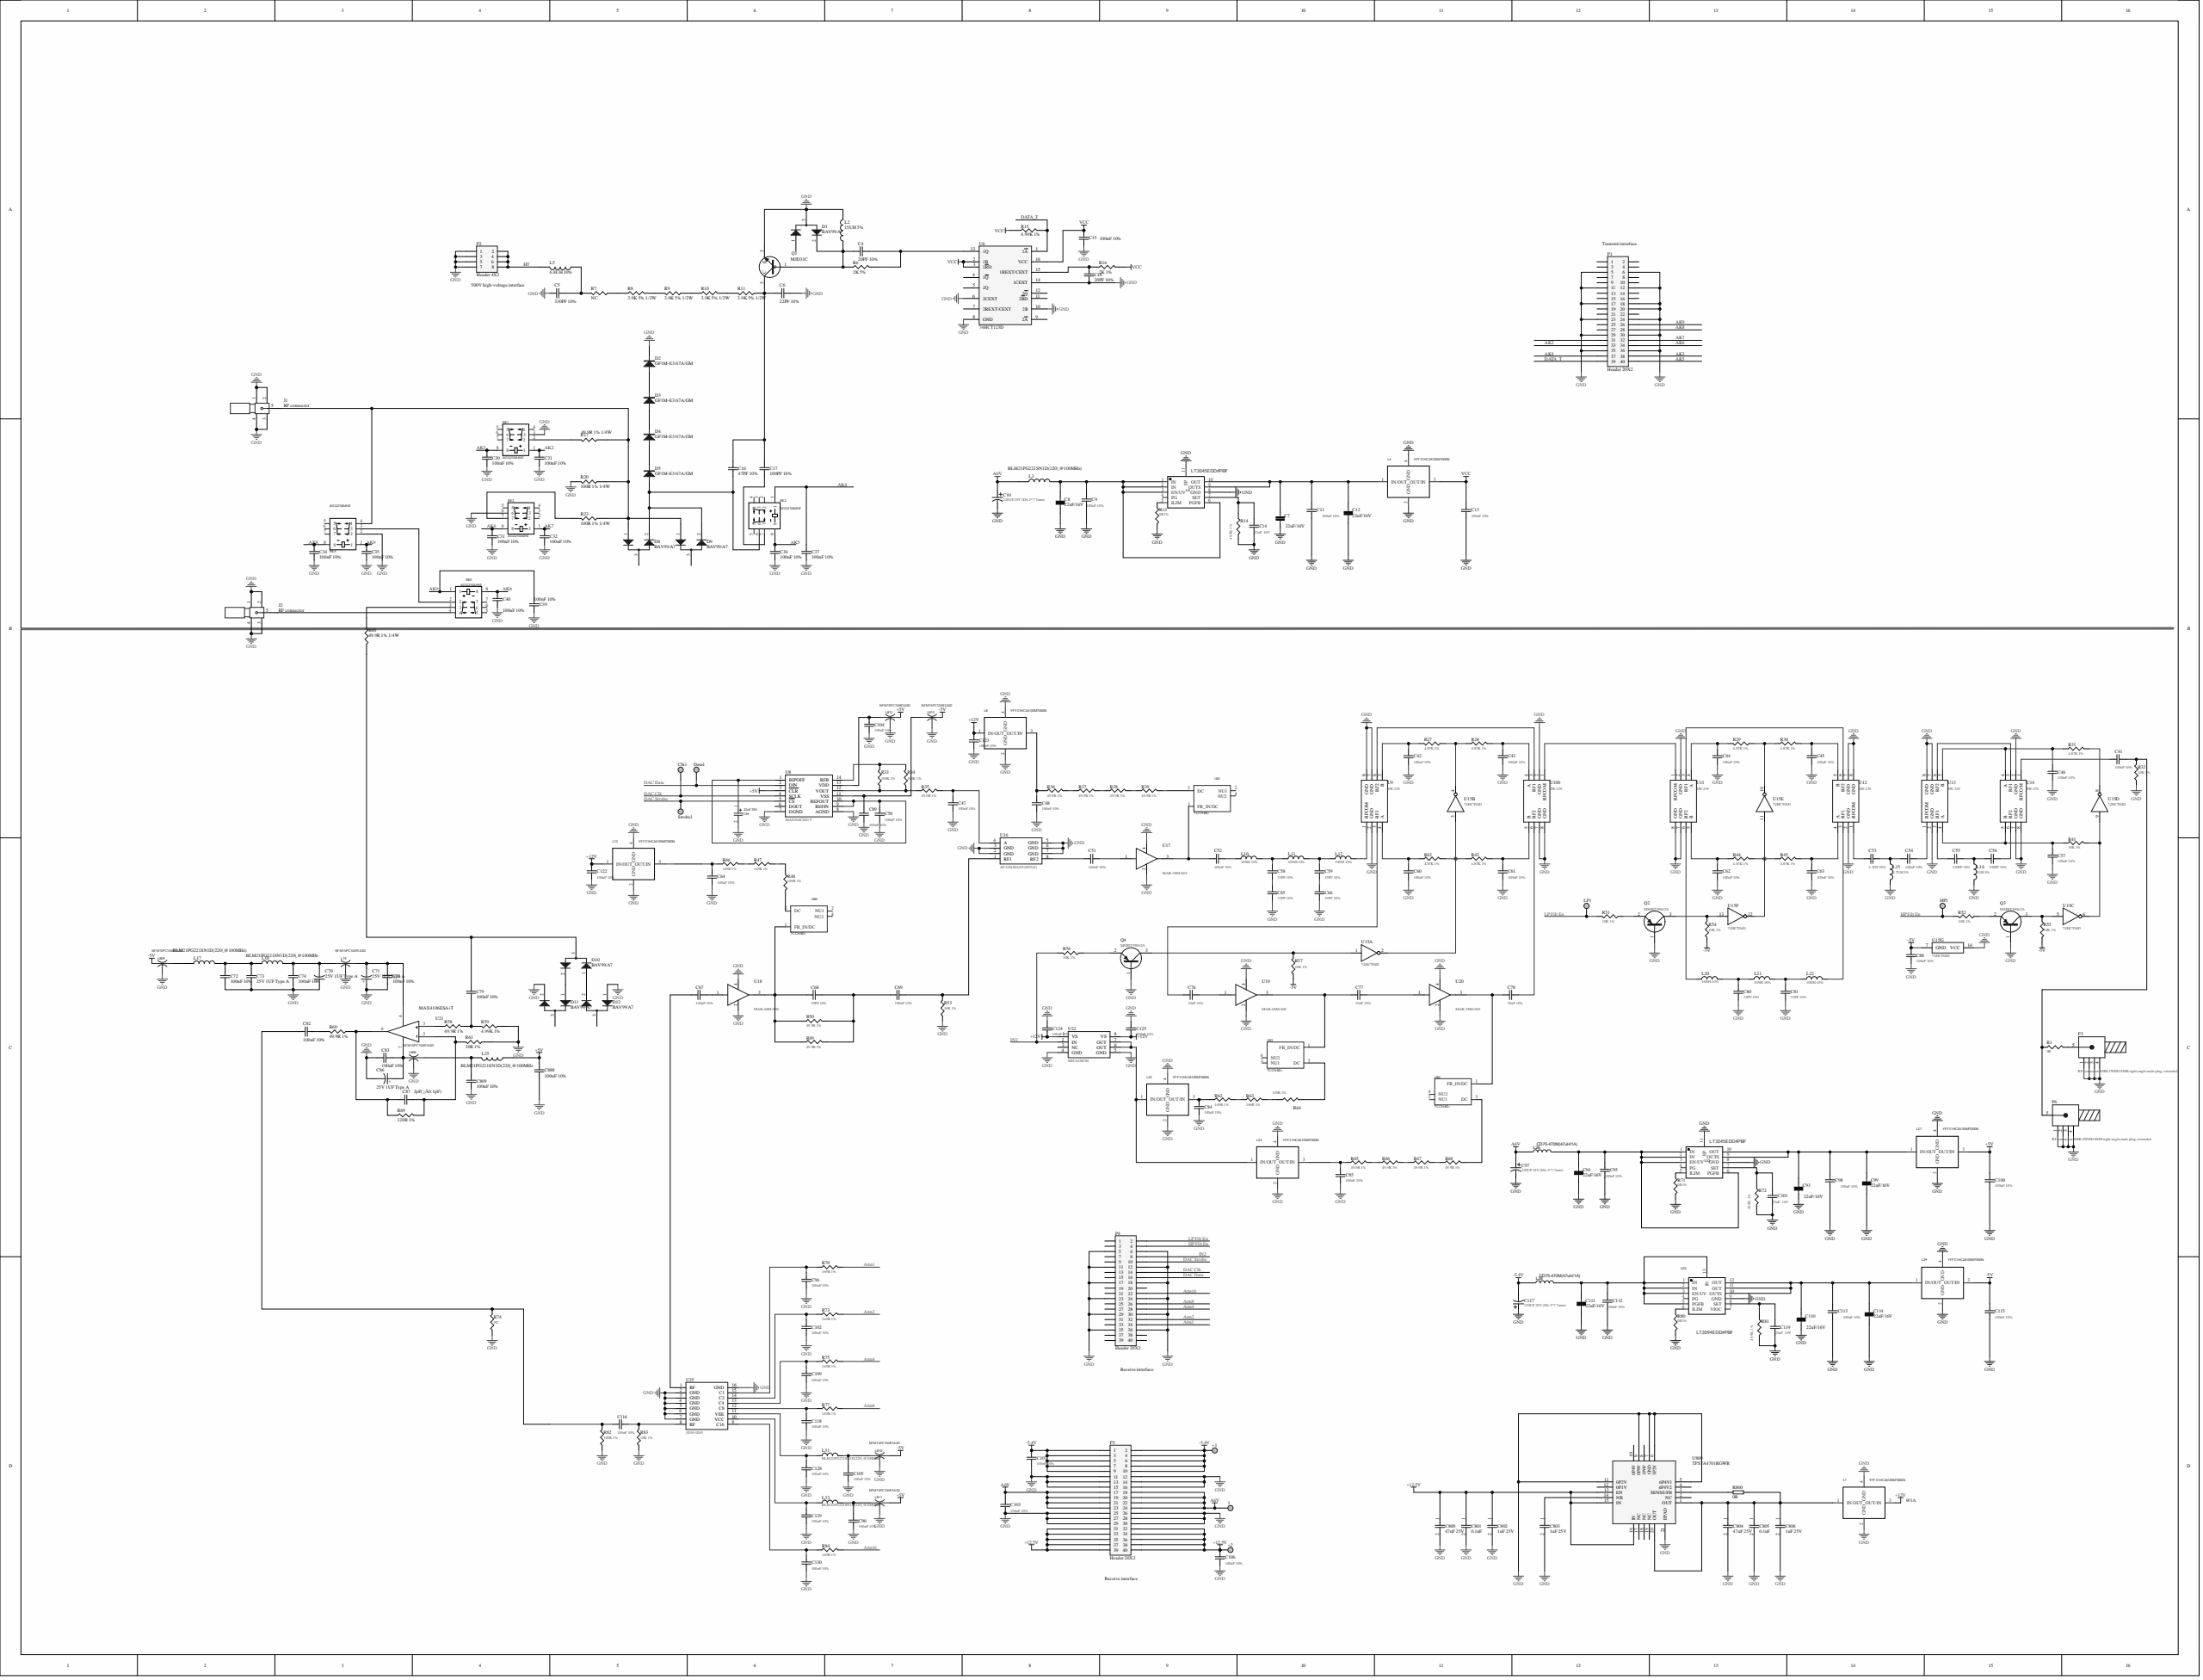Circuit board | Altium Designer | 280 parts | 173 nets
Bill of materials:
Comment,Description,Designator,Footprint,LibRef,Quantity
"","","+1, +2, 1, Clk1, Data1, HP1, LP1, Strobe1","DIP-1","TP","8"
"20PF 10%","Capacitor","C4","0805C-2","CAP","1"
"330PF 10%","Capacitor","C5","1812C","CAP","1"
"22PF 10%","Capacitor","C6","1812C-2","CAP","1"
"22uF/16V","","C7, C8, C12, C93, C94, C99, C110, C111, C114","0805","C1206","9"
"100nF 10%","Capacitor","C9, C11, C95, C98, C112, C113","0603","CAP","6"
"220UF 25V (D6.3*7.7mm)","Capacitor","C10, C97, C117","CAP-SMD_BD6.3-L6.6-W6.6-FD","CAPACITOR_1","3"
"100nF 10%","Capacitor","C13, C15, C20, C21, C31, C32, C34, C35, C36, C37, C39, C40, C41, C42, C43, C44, C45, C46, C47, C48, C50, C51, C52, C54, C57, C60, C61, C62, C63, C64, C67, C69, C72, C74, C75, C82, C83, C84, C85, C88, C89, C90, C96, C100, C102, C103, C104, C105, C106, C107, C109, C115, C116, C118, C122, C123, C124, C125, C128, C129, C130, C809, C888","0805R","CAP","63"
"22uF  16V","Capacitor","C14, C101, C119","0805","CAP","3"
"47PF 10%","Capacitor","C16","1812C-2","CAP","1"
"100PF 10%","Capacitor","C17","1812C-2","CAP","1"
"20PF 10%","Capacitor","C18","0805R","CAP","1"
"22uF 25V","","C49","CAP-SMD_L6.0-W3.2-R-RD","TAJC226K025RNJ","1"
"3.3NF 10%","Capacitor","C53","0805R","CAP","1"
"330PF 10%","Capacitor","C55, C56","0805R","CAP","2"
"33PF 10%","Capacitor","C58, C59, C65, C66, C80, C81","0805R","CAP","6"
"39PF 10%","Capacitor","C68","0805R","CAP","1"
"25V 1UF Type A","Capacitor","C70, C71, C73, C86","0805C-2","CAPACITOR POL, CAP","4"
"10nF 10%","Capacitor","C76, C77, C78","0805R","CAP","3"
"100nF 10%","Capacitor","C79","0603C","CAP","1"
"3pF( ¡À0.1pF)","Capacitor","C87","0805R","CAP","1"
"47uF 25V","Capacitor","C800, C804","1206","CAP","2"
"0.1uF","Capacitor","C801, C805","0402","CAP","2"
"1uF 25V","Capacitor","C802, C803, C806","0402","CAP","3"
"BAV99/A7","","D1","SOT-23","BAV99","1"
"GF1M-E3/67A/GM","Diode","D2, D3, D4, D5","1808D","DIODE","4"
"BAV99/A7","","D8, D9, D10, D11, D12","SOT-23-2","BAV99","5"
"RF connector","","J1, J2","DIP-P","SMA-KWE","2"
"YFF31HC2A105MT000N","","L1, L4, L8, L13, L23, L24, L27, L29","FILTER-SMD_4P-L3.2-W1.6-L_YFF31HC","YFF31HC2A105MT000N","8"
"15UH 5%","","L2","1005R","INDUCTOR","1"
"BLM21PG221SN1D(220|¸@100MHz)","","L3, L17","0805R","INDUCTOR","2"
"6.8UH 10%","","L5","0805R","INDUCTOR","1"
"10NH 10%","","L10, L11, L12, L20, L21, L22","0805R","INDUCTOR","6"
"4.7UH 5%","","L15","1005L","INDUCTOR","1"
"1UH 5%","","L16","0805R","INDUCTOR","1"
"BLM21PG221SN1D(220|¸@100MHz","","L18, L25, L31, L32","0805R","INDUCTOR","4"
"NFM15PC104R1A3D","","L19, L808, L809, L810, L811, L812, L813","FILTER-SMD_0402-3P-L1.0-W0.5-T","NFM15PC104R1A3D","7"
"CD75-470M(47uH/1A)","","L26, L28","IND-SMD_L7.8-W7.0-A","4.7uH/5a","2"
"Header 20X2","Header, 20-Pin, Dual row","P1, P4, P5","N0.8mm/40Pin-Plug","Header 20X2","3"
"Header 4X2","Header, 4-Pin, Dual row","P2","N0.8mm/8Pin-SOCKET","Header 4X2","1"
"RF connector SMB-JWHD SMB right-angle male plug, extended","","P3, P6","DIP-P-2","JA1","2"
"MJD31C","NPN Transistor","Q1","SOT-252-2","NPN","1"
"MMBT3906/2A","PNP Transistor","Q2, Q3, Q4","SOT-23","PNP","3"
"0R","","R1","0805R","RES1","1"
"2K 5%","","R6","0603","RES1","1"
"NC","","R7","AXIAL-0.51","RES1","1"
"3.9K 5% 1/2W","","R8, R9, R10, R11","AXIAL-0.51","RES1","4"
"0R1%","","R13, R71, R80","0603","RES1","3"
"49.9K 1%","","R14, R72, R81","0603","RES1","3"
"4.99K 1%","","R15, R59","0805R","RES1","2"
"2K 1%","","R16","0805R","RES1","1"
"49.9R 1% 1/4W","","R17","AXIAL-0.4","RES1","1"
"100R 1% 1/4W","","R20, R23","AXIAL-0.4","RES1","2"
"4.87K 1%","","R27, R28, R29, R30, R31, R42, R43, R44, R45","0805R","RES1","9"
"10K 1%","","R32, R41, R51, R52, R53, R54, R55, R56, R57, R83","0805R","RES1","10"
"100K 1%","","R33, R34, R82","0805R","RES1","3"
"49.9R 1%","","R35, R36, R37, R38, R39, R49, R50, R58, R65, R66, R67, R68","0805R","RES1","12"
"49.9R 1% 1/4W","","R40","R-SMD_L3.5-W1.5","RES1","1"
"169R 1%","","R46, R47, R48, R62, R63, R64, R70, R73, R75, R77, R84","0805R","RES1","11"
"49.9R 1%","","R60","R-SMD_L3.5-W1.5","RES1","1"
"30R 1%","","R61","R-SMD_L3.5-W1.5","RES1","1"
"120R 1%","","R69","R-SMD_L3.5-W1.5","RES1","1"
"NC","","R74","0805R","RES1","1"
"0R","","R800","0402","RES","1"
"AGQ210A4HZ","","RE1, RE2, RE3, RE4, RE5","RELAY-SMD_PANASONIC_AGQ2X0AXX","AGQ210A4HZ","5"
"LT3045EDD#PBF","","U4, U23","DFN-10_L3.0-W3.0-P0.50-BL-EP","LT3045EDD#PBF","2"
"74HCT123D","","U6","SOIC-16_L9.9-W3.9-P1.27-LS6.0-BL","74HCT123D","1"
"MAX504CSD+T","","U8","SO-14","MAX504CSD+T","1"
"SW-239","","U9, U11, U12, U13, U14, U100","SO-8","SW-239","6"
"74HCT04D","","U15","SO-14","74HC04","1"
"AT-250(MAAV-007941)","","U16","SO-8","AT-250","1"
"MAR-3SM/A03","","U17, U20","LCC4","MAR-3SM","2"
"MAR-6SM/A06","","U18, U19","LCC4","MAR-6SM","2"
"MAX4106ESA+T","","U21","SO-8","MAX4107ESA","1"
"MIC4420CM","","U22","SO-8","MIC4420CM","1"
"LT3094EDD#PBF","","U24","WDFN-12_L3.0-W3.0-P0.45-BL-EP","LT3094EDD#PBF","1"
"AT65-0263","","U25","SO-16","AT65-0263","1"
"TCCH-80+","","U80, U81, U82, U83","IND-SMD_4P-L3.8-W3.8","TCCH-80+","4"
"TPS7A4701RGWR","","U800","QFN-20","TPS7A4701RGWR(QFN20)","1"
Netlist (Protel format):
[
1
DIP-1




]
[
+1
DIP-1




]
[
+2
DIP-1




]
[
C4
0805C-2
20PF 10%



]
[
C5
1812C
330PF 10%



]
[
C6
1812C-2
22PF 10%



]
[
C7
0805
22uF/16V



]
[
C8
0805
22uF/16V



]
[
C9
0603
100nF 10%



]
[
C10
CAP-SMD_BD6.3-L6.6-W6.6-FD
220UF 25V (D6.3*7.7mm)



]
[
C11
0603
100nF 10%



]
[
C12
0805
22uF/16V



]
[
C13
0805R
100nF 10%



]
[
C14
0805
22uF  16V



]
[
C15
0805R
100nF 10%



]
[
C16
1812C-2
47PF 10%



]
[
C17
1812C-2
100PF 10%



]
[
C18
0805R
20PF 10%



]
[
C20
0805R
100nF 10%



]
[
C21
0805R
100nF 10%



]
[
C31
0805R
100nF 10%



]
[
C32
0805R
100nF 10%



]
[
C34
0805R
100nF 10%



]
[
C35
0805R
100nF 10%



]
[
C36
0805R
100nF 10%



]
[
C37
0805R
100nF 10%



]
[
C39
0805R
100nF 10%



]
[
C40
0805R
100nF 10%



]
[
C41
0805R
100nF 10%



]
[
C42
0805R
100nF 10%



]
[
C43
0805R
100nF 10%



]
[
C44
0805R
100nF 10%



]
[
C45
0805R
100nF 10%



]
[
C46
0805R
100nF 10%



]
[
C47
0805R
100nF 10%



]
[
C48
0805R
100nF 10%



]
[
C49
CAP-SMD_L6.0-W3.2-R-RD
22uF 25V



]
[
C50
0805R
100nF 10%



]
[
C51
0805R
100nF 10%



]
[
C52
0805R
100nF 10%



]
[
C53
0805R
3.3NF 10%



]
[
C54
0805R
100nF 10%



]
[
C55
0805R
330PF 10%



]
[
C56
0805R
330PF 10%



]
[
C57
0805R
100nF 10%



]
[
C58
0805R
33PF 10%



]
[
C59
0805R
33PF 10%



]
[
C60
0805R
100nF 10%



]
[
C61
0805R
100nF 10%



]
[
C62
0805R
100nF 10%



]
[
C63
0805R
100nF 10%



]
[
C64
0805R
100nF 10%



]
[
C65
0805R
33PF 10%



]
[
C66
0805R
33PF 10%



]
[
C67
0805R
100nF 10%



]
[
C68
0805R
39PF 10%



]
[
C69
0805R
100nF 10%



]
[
C70
0805C-2
25V 1UF Type A



]
[
C71
0805C-2
25V 1UF Type A



]
[
C72
0805R
100nF 10%



]
[
C73
0805C-2
25V 1UF Type A



]
[
C74
0805R
100nF 10%



]
[
C75
0805R
100nF 10%



]
[
C76
0805R
10nF 10%



]
[
C77
0805R
10nF 10%



]
[
C78
0805R
10nF 10%



]
[
C79
0603C
100nF 10%



]
[
C80
0805R
33PF 10%



]
[
C81
0805R
33PF 10%



]
[
C82
0805R
100nF 10%



]
[
C83
0805R
100nF 10%



]
[
C84
0805R
100nF 10%



]
[
C85
0805R
100nF 10%



]
[
C86
0805C-2
25V 1UF Type A



]
[
C87
0805R
3pF( ¡À0.1pF)



]
[
C88
0805R
100nF 10%



]
[
C89
0805R
100nF 10%



]
[
C90
0805R
100nF 10%



]
[
C93
0805
22uF/16V



]
[
C94
0805
22uF/16V



]
[
C95
0603
100nF 10%



]
[
C96
0805R
100nF 10%



]
[
C97
CAP-SMD_BD6.3-L6.6-W6.6-FD
220UF 25V (D6.3*7.7mm)



]
[
C98
0603
100nF 10%



]
[
C99
0805
22uF/16V



]
[
C100
0805R
100nF 10%



]
[
C101
0805
22uF  16V



]
[
C102
0805R
100nF 10%



]
[
C103
0805R
100nF 10%



]
[
C104
0805R
100nF 10%



]
[
C105
0805R
100nF 10%



]
[
C106
0805R
100nF 10%



]
[
C107
0805R
100nF 10%



]
[
C109
0805R
100nF 10%



]
[
C110
0805
22uF/16V



]
[
C111
0805
22uF/16V



]
[
C112
0603
100nF 10%



]
[
C113
0603
100nF 10%



]
[
C114
0805
22uF/16V



]
[
C115
0805R
100nF 10%



]
[
C116
0805R
100nF 10%



]
[
C117
CAP-SMD_BD6.3-L6.6-W6.6-FD
220UF 25V (D6.3*7.7mm)



]
[
C118
0805R
100nF 10%



]
[
C119
0805
22uF  16V



]
[
C122
0805R
100nF 10%



]
[
C123
0805R
100nF 10%



]
[
C124
0805R
100nF 10%



]
[
C125
0805R
100nF 10%



]
[
C128
0805R
100nF 10%



]
[
C129
0805R
100nF 10%



]
[
C130
0805R
100nF 10%



]
[
C800
1206
47uF 25V



]
[
C801
0402
0.1uF



]
[
C802
0402
1uF 25V



]
[
C803
0402
1uF 25V



]
[
C804
1206
47uF 25V



]
[
C805
0402
0.1uF



]
[
C806
0402
1uF 25V



]
[
C809
0805R
100nF 10%



]
[
C888
0805R
100nF 10%



]
[
Clk1
DIP-1




]
[
D1
SOT-23
BAV99/A7



]
[
D2
1808D
GF1M-E3/67A/GM



]
[
D3
1808D
GF1M-E3/67A/GM



]
[
D4
1808D
GF1M-E3/67A/GM



]
[
D5
1808D
GF1M-E3/67A/GM



]
[
D8
SOT-23-2
BAV99/A7



]
[
D9
SOT-23-2
BAV99/A7



]
[
D10
SOT-23-2
BAV99/A7



]
[
D11
SOT-23-2
BAV99/A7



]
[
D12
SOT-23-2
BAV99/A7



]
[
Data1
DIP-1




]
[
HP1
DIP-1




]
[
J1
DIP-P
RF connector



]
[
J2
DIP-P
RF connector



]
[
L1
FILTER-SMD_4P-L3.2-W1.6-L_YFF31HC
YFF31HC2A105MT000N



]
[
L2
1005R
15UH 5%



]
[
L3
0805R
BLM21PG221SN1D(220|¸@100MHz)



]
[
L4
FILTER-SMD_4P-L3.2-W1.6-L_YFF31HC
YFF31HC2A105MT000N



]
[
L5
0805R
6.8UH 10%



]
[
L8
FILTER-SMD_4P-L3.2-W1.6-L_YFF31HC
YFF31HC2A105MT000N



]
[
L10
0805R
10NH 10%



]
[
L11
0805R
10NH 10%



]
[
L12
0805R
10NH 10%



]
[
L13
FILTER-SMD_4P-L3.2-W1.6-L_YFF31HC
YFF31HC2A105MT000N



]
[
L15
1005L
4.7UH 5%



]
[
L16
0805R
1UH 5%



]
[
L17
0805R
BLM21PG221SN1D(220|¸@100MHz)



]
[
L18
0805R
BLM21PG221SN1D(220|¸@100MHz



]
[
L19
FILTER-SMD_0402-3P-L1.0-W0.5-T
NFM15PC104R1A3D



]
[
L20
0805R
10NH 10%



]
[
L21
0805R
10NH 10%



]
[
L22
0805R
10NH 10%



]
[
L23
FILTER-SMD_4P-L3.2-W1.6-L_YFF31HC
YFF31HC2A105MT000N



]
[
L24
FILTER-SMD_4P-L3.2-W1.6-L_YFF31HC
YFF31HC2A105MT000N



]
[
L25
0805R
BLM21PG221SN1D(220|¸@100MHz



]
[
L26
IND-SMD_L7.8-W7.0-A
CD75-470M(47uH/1A)



]
[
L27
FILTER-SMD_4P-L3.2-W1.6-L_YFF31HC
YFF31HC2A105MT000N



]
[
L28
IND-SMD_L7.8-W7.0-A
CD75-470M(47uH/1A)



]
[
L29
FILTER-SMD_4P-L3.2-W1.6-L_YFF31HC
YFF31HC2A105MT000N



]
[
L31
0805R
BLM21PG221SN1D(220|¸@100MHz



]
[
L32
0805R
BLM21PG221SN1D(220|¸@100MHz



]
[
L808
FILTER-SMD_0402-3P-L1.0-W0.5-T
NFM15PC104R1A3D



]
[
L809
FILTER-SMD_0402-3P-L1.0-W0.5-T
NFM15PC104R1A3D



]
[
L810
FILTER-SMD_0402-3P-L1.0-W0.5-T
NFM15PC104R1A3D



]
[
L811
FILTER-SMD_0402-3P-L1.0-W0.5-T
NFM15PC104R1A3D



]
[
L812
FILTER-SMD_0402-3P-L1.0-W0.5-T
NFM15PC104R1A3D



]
[
L813
FILTER-SMD_0402-3P-L1.0-W0.5-T
NFM15PC104R1A3D



]
[
LP1
DIP-1




]
[
P1
N0.8mm/40Pin-Plug
Header 20X2



]
[
P2
N0.8mm/8Pin-SOCKET
Header 4X2



]
[
P3
DIP-P-2
RF connector SMB-JWHD SMB right-angle male plug, extended



]
[
P4
N0.8mm/40Pin-Plug
Header 20X2



]
[
P5
N0.8mm/40Pin-Plug
Header 20X2



]
[
P6
DIP-P-2
RF connector SMB-JWHD SMB right-angle male plug, extended



]
[
Q1
SOT-252-2
MJD31C



]
[
Q2
SOT-23
MMBT3906/2A



]
[
Q3
SOT-23
MMBT3906/2A



]
[
Q4
SOT-23
MMBT3906/2A



]
[
R1
0805R
0R



]
[
R6
0603
2K 5%



]
[
R7
AXIAL-0.51
NC



]
[
R8
AXIAL-0.51
3.9K 5% 1/2W



]
[
R9
AXIAL-0.51
3.9K 5% 1/2W



]
[
R10
AXIAL-0.51
3.9K 5% 1/2W



]
[
R11
AXIAL-0.51
3.9K 5% 1/2W



]
[
R13
0603
0R1%



]
[
R14
0603
49.9K 1%



]
[
R15
0805R
4.99K 1%



]
[
R16
0805R
2K 1%



]
[
R17
AXIAL-0.4
49.9R 1% 1/4W



]
[
R20
AXIAL-0.4
100R 1% 1/4W



]
[
R23
AXIAL-0.4
100R 1% 1/4W



]
[
R27
0805R
4.87K 1%



]
[
R28
0805R
4.87K 1%



]
[
R29
0805R
4.87K 1%



]
[
R30
0805R
4.87K 1%



]
[
R31
0805R
4.87K 1%



]
[
R32
0805R
10K 1%



]
[
R33
0805R
100K 1%



]
[
R34
0805R
100K 1%



]
[
R35
0805R
49.9R 1%



]
[
R36
0805R
49.9R 1%



]
[
R37
0805R
49.9R 1%



]
[
R38
0805R
49.9R 1%



]
[
R39
0805R
49.9R 1%



]
[
R40
R-SMD_L3.5-W1.5
49.9R 1% 1/4W



]
[
R41
0805R
10K 1%



]
[
R42
0805R
4.87K 1%



]
[
R43
0805R
4.87K 1%



]
[
R44
0805R
4.87K 1%



]
[
R45
0805R
4.87K 1%



]
[
R46
0805R
169R 1%



]
[
R47
0805R
169R 1%



]
[
R48
0805R
169R 1%



]
[
R49
0805R
49.9R 1%



]
[
R50
0805R
49.9R 1%



]
[
R51
0805R
10K 1%



]
[
R52
0805R
10K 1%



]
[
R53
0805R
10K 1%



]
[
R54
0805R
10K 1%



]
[
R55
0805R
10K 1%



]
[
R56
0805R
10K 1%



]
[
R57
0805R
10K 1%



]
[
R58
0805R
49.9R 1%



]
[
R59
0805R
4.99K 1%



]
[
R60
R-SMD_L3.5-W1.5
49.9R 1%



]
[
R61
R-SMD_L3.5-W1.5
30R 1%



]
[
R62
0805R
169R 1%



]
[
R63
0805R
169R 1%



]
[
R64
0805R
169R 1%



]
[
R65
0805R
49.9R 1%



]
[
R66
0805R
49.9R 1%



]
[
R67
0805R
49.9R 1%



]
[
R68
0805R
49.9R 1%



]
[
R69
R-SMD_L3.5-W1.5
120R 1%



]
[
R70
0805R
169R 1%



]
[
R71
0603
0R1%



]
[
R72
0603
49.9K 1%



]
[
R73
0805R
169R 1%



]
[
R74
0805R
NC



]
[
R75
0805R
169R 1%



]
[
R77
0805R
169R 1%



]
[
R80
0603
0R1%



]
[
R81
0603
49.9K 1%



]
[
R82
0805R
100K 1%



]
[
R83
0805R
10K 1%



]
[
R84
0805R
169R 1%



]
[
R800
0402
0R



]
[
RE1
RELAY-SMD_PANASONIC_AGQ2X0AXX
AGQ210A4HZ



]
[
RE2
RELAY-SMD_PANASONIC_AGQ2X0AXX
AGQ210A4HZ



]
[
RE3
RELAY-SMD_PANASONIC_AGQ2X0AXX
AGQ210A4HZ



]
[
RE4
RELAY-SMD_PANASONIC_AGQ2X0AXX
AGQ210A4HZ



]
[
RE5
RELAY-SMD_PANASONIC_AGQ2X0AXX
AGQ210A4HZ



]
[
Strobe1
DIP-1




]
[
U4
DFN-10_L3.0-W3.0-P0.50-BL-EP
LT3045EDD#PBF



]
[
U6
SOIC-16_L9.9-W3.9-P1.27-LS6.0-BL
74HCT123D



]
[
U8
SO-14
MAX504CSD+T



]
[
U9
SO-8
SW-239



]
[
U11
SO-8
SW-239



]
[
U12
SO-8
SW-239



]
[
U13
SO-8
SW-239



]
[
U14
SO-8
SW-239



]
[
U15
SO-14
74HCT04D



]
[
U16
SO-8
AT-250(MAAV-007941)



]
[
U17
LCC4
MAR-3SM/A03



]
[
U18
LCC4
MAR-6SM/A06



]
[
U19
LCC4
MAR-6SM/A06



]
[
U20
LCC4
MAR-3SM/A03



]
[
U21
SO-8
MAX4106ESA+T



]
[
U22
SO-8
MIC4420CM



]
[
U23
DFN-10_L3.0-W3.0-P0.50-BL-EP
LT3045EDD#PBF



]
[
U24
WDFN-12_L3.0-W3.0-P0.45-BL-EP
LT3094EDD#PBF



]
[
U25
SO-16
AT65-0263



]
[
U80
IND-SMD_4P-L3.8-W3.8
TCCH-80+



]
[
U81
IND-SMD_4P-L3.8-W3.8
TCCH-80+



]
[
U82
IND-SMD_4P-L3.8-W3.8
TCCH-80+



]
[
U83
IND-SMD_4P-L3.8-W3.8
TCCH-80+



]
[
U100
SO-8
SW-239



]
[
U800
QFN-20
TPS7A4701RGWR



]
(
VCC
C13-1
C15-2
L4-3
R15-1
R16-2
U6-2
U6-3
U6-16
)
(
NetU13_6
U13-6
U14-3
)
(
NetU11_3
U11-3
U12-6
)
(
NetU11_1
U11-1
U100-1
)
(
NetU9_6
U9-6
U100-3
)
(
NetRE4_3
RE4-3
RE5-2
)
(
NetR800_2
R800-2
U800-3
)
(
NetR80_1
R80-1
U24-6
)
(
NetR71_1
R71-1
U23-5
)
(
NetR68_2
R68-2
U82-3
)
(
NetR67_2
R67-2
R68-1
)
(
NetR66_1
R66-1
R67-1
)
(
NetR65_2
R65-2
R66-2
)
(
NetR64_1
R64-1
U83-3
)
(
NetR63_2
R63-2
R64-2
)
(
NetR62_1
R62-1
R63-1
)
(
NetR58_1
R58-1
U21-3
)
(
NetR48_2
R48-2
U80-3
)
(
NetR47_1
R47-1
R48-1
)
(
NetR46_1
R46-1
R47-2
)
(
NetR44_2
R44-2
R45-2
U15-11
U15-12
)
(
NetR42_2
R42-2
R43-1
U15-2
U15-3
)
(
NetR41_2
R41-2
U15-6
U15-9
)
(
NetR40_1
R40-1
RE5-3
)
(
NetR39_2
R39-2
U81-3
)
(
NetR38_1
R38-1
R39-1
)
(
NetR37_2
R37-2
R38-2
)
(
NetR36_2
R36-2
R37-1
)
(
NetR33_2
R33-2
R34-2
R35-2
U8-12
)
(
NetR33_1
R33-1
R34-1
U8-14
)
(
NetR31_2
R31-2
U15-8
)
(
NetR29_2
R29-2
R30-2
U15-10
)
(
NetR27_2
R27-2
R28-1
U15-4
)
(
NetR23_2
R23-2
RE3-7
)
(
NetR17_2
R17-2
RE1-2
)
(
NetR13_1
R13-1
U4-5
)
(
NetR10_2
R10-2
R11-2
)
(
NetR9_1
R9-1
R10-1
)
(
NetR8_2
R8-2
R9-2
)
(
NetR7_1
R7-1
R8-1
)
(
NetQ4_3
Q4-3
R57-2
U15-1
)
(
NetQ4_2
Q4-2
R56-2
)
(
NetQ3_3
Q3-3
R55-1
U15-5
)
(
NetQ3_2
Q3-2
R52-1
)
(
NetQ2_3
Q2-3
R54-2
U15-13
)
(
NetQ2_2
Q2-2
R51-1
)
(
NetP3_5
P3-5
R1-2
)
(
NetL23_1
L23-1
L24-1
U22-6
U22-7
)
(
NetL22_2
L22-2
U12-3
)
(
NetL20_1
L20-1
U11-6
)
(
NetL17_1
L17-1
L809-3
)
(
NetL12_2
L12-2
U9-1
)
(
NetJ2_5
J2-5
RE5-4
)
(
NetD10_2
D10-2
D11-1
)
(
NetD10_1
D10-1
D12-2
)
(
NetD8_1
D8-1
D9-1
J1-5
R17-1
R20-1
R23-1
RE4-4
)
(
NetD4_1
D4-1
D5-2
)
(
NetD3_1
D3-1
D4-2
)
(
NetD2_1
D2-1
D3-2
)
(
NetC809_1
C809-1
L25-2
L808-3
)
(
NetC804_1
C804-1
C805-1
C806-1
L1-1
R800-1
U800-1
U800-20
)
(
NetC803_1
C803-1
U800-14
)
(
NetC130_1
C130-1
R84-1
U25-9
)
(
NetC129_2
C129-2
L32-1
U25-10
)
(
NetC128_2
C128-2
L31-2
U25-11
)
(
NetC119_1
C119-1
R81-1
U24-8
)
(
NetC118_1
C118-1
R77-1
U25-12
)
(
NetC116_2
C116-2
R83-2
U25-8
)
(
NetC111_2
C111-2
C112-1
L28-1
U24-1
U24-2
U24-3
U24-5
U24-13
)
(
NetC110_2
C110-2
C113-1
C114-2
L29-1
U24-10
U24-11
U24-12
)
(
NetC109_1
C109-1
R75-1
U25-13
)
(
NetC105_2
C105-2
L31-1
L810-1
)
(
NetC104_1
C104-1
L812-1
U8-13
)
(
NetC102_1
C102-1
R73-1
U25-14
)
(
NetC101_1
C101-1
R72-1
U23-7
)
(
NetC96_1
C96-1
R70-1
U25-15
)
(
NetC94_2
C94-2
C95-1
L26-1
U23-1
U23-2
U23-3
U23-6
)
(
NetC93_2
C93-2
C98-1
C99-2
L27-1
U23-9
U23-10
)
(
NetC90_1
C90-1
L32-2
L811-1
)
(
NetC89_1
C89-1
L813-1
U8-11
)
(
NetC87_2
C87-2
R61-2
R69-2
U21-2
)
(
NetC87_1
C87-1
R60-1
R69-1
U21-6
)
(
NetC85_2
C85-2
L24-3
R65-1
)
(
NetC84_1
C84-1
L23-3
R62-2
)
(
NetC83_1
C83-1
C86-1
L808-1
U21-7
)
(
NetC82_2
C82-2
C116-1
R74-2
R82-2
)
(
NetC82_1
C82-1
R60-2
)
(
NetC81_2
C81-2
L21-1
L22-1
)
(
NetC80_2
C80-2
L20-2
L21-2
)
(
NetC79_2
C79-2
R58-2
R59-2
)
(
NetC79_1
C79-1
D10-3
R40-2
)
(
NetC78_2
C78-2
U100-6
)
(
NetC78_1
C78-1
U20-3
U82-1
)
(
NetC77_2
C77-2
U20-1
)
(
NetC77_1
C77-1
U19-3
U83-1
)
(
NetC76_2
C76-2
U19-1
)
(
NetC76_1
C76-1
U9-3
)
(
NetC72_1
C72-1
C73-2
L17-2
L18-2
)
(
NetC71_2
C71-2
C75-2
L19-3
U21-4
)
(
NetC70_2
C70-2
C74-2
L18-1
L19-1
)
(
NetC69_1
C69-1
R53-2
U16-1
)
(
NetC68_2
C68-2
R49-1
R50-1
U18-3
U80-1
)
(
NetC68_1
C68-1
C69-2
R49-2
R50-2
)
(
NetC67_2
C67-2
U25-1
)
(
NetC67_1
C67-1
U18-1
)
(
NetC64_2
C64-2
L13-3
R46-2
)
(
NetC63_2
C63-2
R45-1
U12-4
)
(
NetC62_2
C62-2
R44-1
U11-5
)
(
NetC61_2
C61-2
R43-2
U100-5
)
(
NetC60_1
C60-1
R42-1
U9-4
)
(
NetC59_2
C59-2
C66-2
)
(
NetC59_1
C59-1
L11-2
L12-1
)
(
NetC58_2
C58-2
L10-1
L11-1
)
(
NetC58_1
C58-1
C65-1
)
(
NetC57_1
C57-1
R41-1
U13-4
U14-5
)
(
NetC56_2
C56-2
U14-6
)
(
NetC55_2
C55-2
C56-1
L16-2
)
(
NetC55_1
C55-1
U13-3
)
(
NetC54_2
C54-2
U13-1
)
(
NetC53_2
C53-2
U12-1
)
(
NetC53_1
C53-1
C54-1
L15-1
)
(
NetC52_2
C52-2
U17-3
U81-1
)
(
NetC52_1
C52-1
L10-2
)
(
NetC51_2
C51-2
U16-8
)
(
NetC51_1
C51-1
U17-1
)
(
NetC49_1
C49-1
C50-1
U8-1
U8-9
U8-10
)
(
NetC48_2
C48-2
L8-3
R36-1
)
(
NetC47_2
C47-2
R35-1
U16-4
)
(
NetC46_1
C46-1
R31-1
U13-5
U14-4
)
(
NetC45_1
C45-1
R30-1
U12-5
)
(
NetC44_1
C44-1
R29-1
U11-4
)
(
NetC43_2
C43-2
R28-2
U100-4
)
(
NetC42_1
C42-1
R27-1
U9-5
)
(
NetC41_2
C41-2
P6-5
R1-1
R32-1
)
(
NetC41_1
C41-1
U14-1
)
(
NetC18_1
C18-1
R16-1
U6-15
)
(
NetC17_1
C17-1
RE2-7
)
(
NetC16_1
C16-1
D5-1
D8-2
D9-2
RE2-6
)
(
NetC14_1
C14-1
R14-1
U4-7
)
(
NetC8_2
C8-2
C9-1
L3-2
U4-1
U4-2
U4-3
U4-6
)
(
NetC7_2
C7-2
C11-1
C12-2
L4-1
U4-9
U4-10
)
(
NetC6_1
C6-1
C16-2
C17-2
Q1-3
R11-1
)
(
NetC5_2
C5-2
L5-2
R7-2
)
(
NetC4_2
C4-2
R6-2
U6-13
)
(
NetC4_1
C4-1
D1-2
L2-1
Q1-1
R6-1
)
(
LP Filt En
LP1-1
P4-2
R51-2
)
(
IN2
P4-8
R56-1
U22-2
)
(
HT
L5-1
P2-2
P2-4
P2-6
P2-8
)
(
HP Filt En
HP1-1
P4-4
R52-2
)
(
GND
C5-1
C6-2
C7-1
C8-1
C9-2
C10-2
C11-2
C12-1
C13-2
C14-2
C15-1
C18-2
C20-1
C21-1
C31-1
C32-1
C34-1
C35-1
C36-2
C37-2
C39-2
C40-2
C42-2
C43-1
C44-2
C45-2
C46-2
C47-1
C48-1
C49-2
C50-2
C57-2
C60-2
C61-1
C62-1
C63-1
C64-1
C65-2
C66-1
C70-1
C71-1
C72-2
C73-1
C74-1
C75-1
C80-1
C81-1
C83-2
C84-2
C85-1
C86-2
C88-1
C89-2
C90-2
C93-1
C94-1
C95-2
C96-2
C97-2
C98-2
C99-1
C100-2
C101-2
C102-2
C103-1
C104-2
C105-1
C106-2
C107-2
C109-2
C110-1
C111-1
C112-2
C113-2
C114-1
C115-1
C117-1
C118-2
C119-2
C122-2
C123-2
C124-1
C125-1
C128-1
C129-1
C130-2
C800-2
C801-2
C802-2
C803-2
C804-2
C805-2
C806-2
C809-2
C888-2
D1-3
D2-2
D11-2
D12-1
J1-1
J1-2
J1-3
J1-4
J2-1
J2-2
J2-3
J2-4
L1-2
L1-4
L2-2
L4-2
L4-4
L8-2
L8-4
L13-2
L13-4
L15-2
L16-1
L19-2
L23-2
L23-4
L24-2
L24-4
L27-2
L27-4
L29-2
L29-4
L808-2
L809-2
L810-2
L811-2
L812-2
L813-2
P1-5
P1-6
P1-11
P1-12
P1-17
P1-18
P1-20
P1-23
P1-24
P1-29
P1-30
P1-35
P1-36
P2-1
P2-3
P2-5
P2-7
P3-1
P3-2
P3-3
P3-4
P4-5
P4-6
P4-11
P4-12
P4-17
P4-18
P4-23
P4-24
P4-29
P4-30
P4-35
P4-36
P5-11
P5-12
P5-13
P5-14
P5-15
P5-16
P5-25
P5-26
P5-27
P5-28
P5-29
P5-30
P6-1
P6-2
P6-3
P6-4
Q1-2
Q2-1
Q3-1
Q4-1
R13-2
R14-2
R20-2
R32-2
R53-1
R59-1
R61-1
R71-2
R72-2
R74-1
R80-2
R81-2
R82-1
R83-1
RE1-3
RE3-6
RE4-2
U4-8
U4-11
U6-6
U6-8
U6-10
U6-14
U8-7
U8-8
U9-2
U9-7
U9-8
U11-2
U11-7
U11-8
U12-2
U12-7
U12-8
U13-2
U13-7
U13-8
U14-2
U14-7
U14-8
U15-14
U16-2
U16-3
U16-5
U16-6
U16-7
U17-2
U17-4
U18-2
U18-4
U19-2
U19-4
U20-2
U20-4
U22-4
U22-5
U23-8
U23-11
U24-9
U25-2
U25-3
U25-4
U25-5
U25-6
U25-7
U25-16
U100-2
U100-7
U100-8
U800-5
U800-6
U800-7
U800-9
U800-11
U800-21
)
(
DATA_T
P1-39
R15-2
U6-1
)
(
DAC Strobe
P4-10
Strobe1-1
U8-5
)
(
DAC Data
Data1-1
P4-16
U8-2
)
(
DAC Clk
Clk1-1
P4-14
U8-4
)
(
Attn16
P4-22
R84-2
)
(
Attn8
P4-26
R77-2
)
(
Attn4
P4-28
R75-2
)
(
Attn2
P4-32
R73-2
)
(
Attn1
P4-34
R70-2
)
(
AK9
C35-2
C39-1
P1-26
RE4-1
RE5-1
)
(
AK8
C34-2
C40-1
P1-28
RE4-8
RE5-8
)
(
AK7
C32-2
P1-32
RE3-1
)
(
AK6
C31-2
P1-34
RE3-8
)
(
AK5
C36-1
P1-40
RE2-8
)
(
AK4
C37-1
P1-37
RE2-1
)
(
AK3
C20-2
P1-38
RE1-8
)
(
AK2
C21-2
P1-33
RE1-1
)
(
A6V
1-1
C10-1
C97-1
C103-2
L3-1
L26-2
P5-17
P5-18
P5-19
P5-20
P5-21
P5-22
P5-23
P5-24
)
(
-5V
C88-2
C115-2
L29-3
L809-1
L810-3
L813-3
R54-1
R55-2
R57-1
U15-7
)
(
-5.4V
+1-1
C107-1
C117-2
L28-2
P5-1
P5-2
P5-3
P5-4
P5-5
P5-6
P5-7
P5-8
P5-9
P5-10
)
(
+12V
C122-1
C123-1
C124-2
C125-2
L1-3
L8-1
L13-1
U22-1
U22-8
)
(
+12.5V
+2-1
C106-1
C800-1
C801-1
C802-1
P5-31
P5-32
P5-33
P5-34
P5-35
P5-36
P5-37
P5-38
P5-39
P5-40
U800-13
U800-15
U800-16
)
(
+5V
C100-1
C888-1
L25-1
L27-3
L811-3
L812-3
U8-3
)